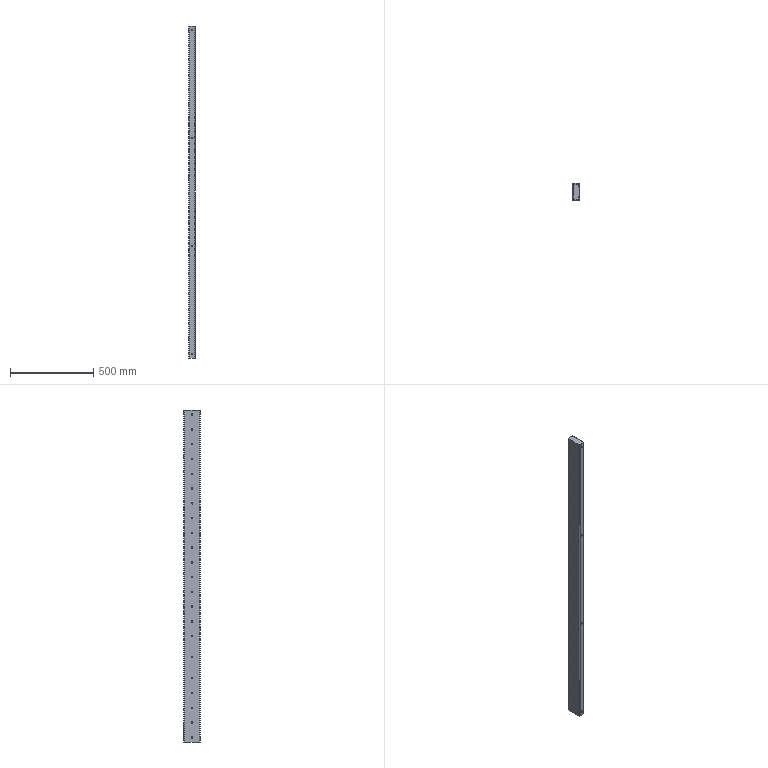Part | SolidWorks | features BaseBody 1 | 1 solid | 99 faces | box 40 x 100 x 2000 mm | volume 1606592 mm3 | cylinder 84 | plane 15 | commonest cylinder face diameters 9 x76 2 x4 10 x4